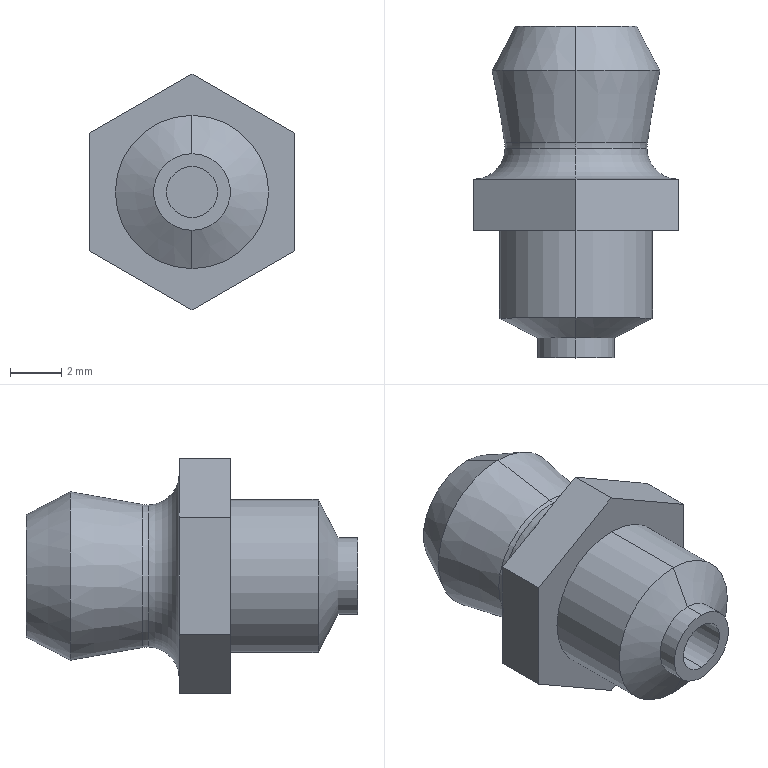Part | STEP file | JB/T7940.1-1995 straight-through grease cup 6 | 1 solid | 35 faces | box 8 x 13 x 9.238 mm | volume 360.504 mm3 | plane 17 | cylinder 8 | cone 6 | torus 4 | commonest cylinder face diameters 2 x4 3 x2 6 x2
STEP:
#1=CARTESIAN_POINT('',(0.,8.43,2.8));
#2=VERTEX_POINT('',#1);
#3=CARTESIAN_POINT('',(0.,8.218,2.782));
#4=VERTEX_POINT('',#3);
#5=CARTESIAN_POINT('',(0.,8.218,4.));
#6=DIRECTION('',(-1.,0.,0.));
#7=DIRECTION('',(0.,0.,1.));
#8=AXIS2_PLACEMENT_3D('',#5,#6,#7);
#9=CIRCLE('',#8,1.218);
#10=EDGE_CURVE('',#2,#4,#9,.T.);
#11=ORIENTED_EDGE('',*,*,#10,.T.);
#12=CARTESIAN_POINT('',(0.,8.218,-2.782));
#13=VERTEX_POINT('',#12);
#14=CARTESIAN_POINT('',(0.,8.218,0.));
#15=DIRECTION('',(0.,1.,0.));
#16=DIRECTION('',(0.,0.,1.));
#17=AXIS2_PLACEMENT_3D('',#14,#15,#16);
#18=CIRCLE('',#17,2.782);
#19=EDGE_CURVE('',#4,#13,#18,.T.);
#20=ORIENTED_EDGE('',*,*,#19,.T.);
#21=CARTESIAN_POINT('',(0.,8.43,-2.8));
#22=VERTEX_POINT('',#21);
#23=CARTESIAN_POINT('',(0.,8.218,-4.));
#24=DIRECTION('',(1.,0.,0.));
#25=DIRECTION('',(0.,0.,-1.));
#26=AXIS2_PLACEMENT_3D('',#23,#24,#25);
#27=CIRCLE('',#26,1.218);
#28=EDGE_CURVE('',#22,#13,#27,.T.);
#29=ORIENTED_EDGE('',*,*,#28,.F.);
#30=CARTESIAN_POINT('',(0.,8.43,0.));
#31=DIRECTION('',(0.,1.,0.));
#32=DIRECTION('',(0.,0.,1.));
#33=AXIS2_PLACEMENT_3D('',#30,#31,#32);
#34=CIRCLE('',#33,2.8);
#35=EDGE_CURVE('',#2,#22,#34,.T.);
#36=ORIENTED_EDGE('',*,*,#35,.F.);
#37=EDGE_LOOP('',(#11,#20,#29,#36));
#38=FACE_OUTER_BOUND('',#37,.T.);
#39=CARTESIAN_POINT('',(0.,8.218,0.));
#40=DIRECTION('',(0.,1.,0.));
#41=DIRECTION('',(0.,0.,1.));
#42=AXIS2_PLACEMENT_3D('',#39,#40,#41);
#43=TOROIDAL_SURFACE('',#42,4.,1.218);
#44=ADVANCED_FACE('',(#38),#43,.F.);
#45=ORIENTED_EDGE('',*,*,#28,.T.);
#46=CARTESIAN_POINT('',(0.,8.218,0.));
#47=DIRECTION('',(0.,1.,0.));
#48=DIRECTION('',(0.,0.,1.));
#49=AXIS2_PLACEMENT_3D('',#46,#47,#48);
#50=CIRCLE('',#49,2.782);
#51=EDGE_CURVE('',#13,#4,#50,.T.);
#52=ORIENTED_EDGE('',*,*,#51,.T.);
#53=ORIENTED_EDGE('',*,*,#10,.F.);
#54=CARTESIAN_POINT('',(0.,8.43,0.));
#55=DIRECTION('',(0.,1.,0.));
#56=DIRECTION('',(0.,0.,1.));
#57=AXIS2_PLACEMENT_3D('',#54,#55,#56);
#58=CIRCLE('',#57,2.8);
#59=EDGE_CURVE('',#22,#2,#58,.T.);
#60=ORIENTED_EDGE('',*,*,#59,.F.);
#61=EDGE_LOOP('',(#45,#52,#53,#60));
#62=FACE_OUTER_BOUND('',#61,.T.);
#63=CARTESIAN_POINT('',(0.,8.218,0.));
#64=DIRECTION('',(0.,1.,0.));
#65=DIRECTION('',(0.,0.,1.));
#66=AXIS2_PLACEMENT_3D('',#63,#64,#65);
#67=TOROIDAL_SURFACE('',#66,4.,1.218);
#68=ADVANCED_FACE('',(#62),#67,.F.);
#69=ORIENTED_EDGE('',*,*,#51,.F.);
#70=CARTESIAN_POINT('',(0.,7.,-4.));
#71=VERTEX_POINT('',#70);
#72=CARTESIAN_POINT('',(0.,8.218,-4.));
#73=DIRECTION('',(1.,0.,0.));
#74=DIRECTION('',(0.,0.,-1.));
#75=AXIS2_PLACEMENT_3D('',#72,#73,#74);
#76=CIRCLE('',#75,1.218);
#77=EDGE_CURVE('',#13,#71,#76,.T.);
#78=ORIENTED_EDGE('',*,*,#77,.T.);
#79=CARTESIAN_POINT('',(-2.,7.,-3.464));
#80=VERTEX_POINT('',#79);
#81=CARTESIAN_POINT('',(0.,7.,0.));
#82=DIRECTION('',(0.,1.,0.));
#83=DIRECTION('',(0.,0.,1.));
#84=AXIS2_PLACEMENT_3D('',#81,#82,#83);
#85=CIRCLE('',#84,4.);
#86=EDGE_CURVE('',#71,#80,#85,.T.);
#87=ORIENTED_EDGE('',*,*,#86,.T.);
#88=CARTESIAN_POINT('',(-4.,7.,0.));
#89=VERTEX_POINT('',#88);
#90=CARTESIAN_POINT('',(0.,7.,0.));
#91=DIRECTION('',(0.,1.,0.));
#92=DIRECTION('',(0.,0.,1.));
#93=AXIS2_PLACEMENT_3D('',#90,#91,#92);
#94=CIRCLE('',#93,4.);
#95=EDGE_CURVE('',#80,#89,#94,.T.);
#96=ORIENTED_EDGE('',*,*,#95,.T.);
#97=CARTESIAN_POINT('',(-2.,7.,3.464));
#98=VERTEX_POINT('',#97);
#99=CARTESIAN_POINT('',(0.,7.,0.));
#100=DIRECTION('',(0.,1.,0.));
#101=DIRECTION('',(0.,0.,1.));
#102=AXIS2_PLACEMENT_3D('',#99,#100,#101);
#103=CIRCLE('',#102,4.);
#104=EDGE_CURVE('',#89,#98,#103,.T.);
#105=ORIENTED_EDGE('',*,*,#104,.T.);
#106=CARTESIAN_POINT('',(0.,7.,4.));
#107=VERTEX_POINT('',#106);
#108=CARTESIAN_POINT('',(0.,7.,0.));
#109=DIRECTION('',(0.,1.,0.));
#110=DIRECTION('',(0.,0.,1.));
#111=AXIS2_PLACEMENT_3D('',#108,#109,#110);
#112=CIRCLE('',#111,4.);
#113=EDGE_CURVE('',#98,#107,#112,.T.);
#114=ORIENTED_EDGE('',*,*,#113,.T.);
#115=CARTESIAN_POINT('',(0.,8.218,4.));
#116=DIRECTION('',(-1.,0.,0.));
#117=DIRECTION('',(0.,0.,1.));
#118=AXIS2_PLACEMENT_3D('',#115,#116,#117);
#119=CIRCLE('',#118,1.218);
#120=EDGE_CURVE('',#4,#107,#119,.T.);
#121=ORIENTED_EDGE('',*,*,#120,.F.);
#122=EDGE_LOOP('',(#69,#78,#87,#96,#105,#114,#121));
#123=FACE_OUTER_BOUND('',#122,.T.);
#124=CARTESIAN_POINT('',(0.,8.218,0.));
#125=DIRECTION('',(0.,1.,0.));
#126=DIRECTION('',(0.,0.,1.));
#127=AXIS2_PLACEMENT_3D('',#124,#125,#126);
#128=TOROIDAL_SURFACE('',#127,4.,1.218);
#129=ADVANCED_FACE('',(#123),#128,.F.);
#130=ORIENTED_EDGE('',*,*,#35,.T.);
#131=CARTESIAN_POINT('',(0.,11.271,-3.3));
#132=VERTEX_POINT('',#131);
#133=CARTESIAN_POINT('',(0.,11.271,-3.3));
#134=DIRECTION('',(0.,0.9849,-0.1733));
#135=VECTOR('',#134,1000.);
#136=LINE('',#133,#135);
#137=EDGE_CURVE('',#22,#132,#136,.T.);
#138=ORIENTED_EDGE('',*,*,#137,.T.);
#139=CARTESIAN_POINT('',(0.,11.271,3.3));
#140=VERTEX_POINT('',#139);
#141=CARTESIAN_POINT('',(0.,11.271,0.));
#142=DIRECTION('',(0.,1.,0.));
#143=DIRECTION('',(0.,0.,1.));
#144=AXIS2_PLACEMENT_3D('',#141,#142,#143);
#145=CIRCLE('',#144,3.3);
#146=EDGE_CURVE('',#140,#132,#145,.T.);
#147=ORIENTED_EDGE('',*,*,#146,.F.);
#148=CARTESIAN_POINT('',(0.,11.271,3.3));
#149=DIRECTION('',(0.,0.9849,0.1733));
#150=VECTOR('',#149,1000.);
#151=LINE('',#148,#150);
#152=EDGE_CURVE('',#2,#140,#151,.T.);
#153=ORIENTED_EDGE('',*,*,#152,.F.);
#154=EDGE_LOOP('',(#130,#138,#147,#153));
#155=FACE_OUTER_BOUND('',#154,.T.);
#156=CARTESIAN_POINT('',(0.,11.271,0.));
#157=DIRECTION('',(0.,1.,0.));
#158=DIRECTION('',(0.,0.,1.));
#159=AXIS2_PLACEMENT_3D('',#156,#157,#158);
#160=CONICAL_SURFACE('',#159,3.3,0.1742);
#161=ADVANCED_FACE('',(#155),#160,.T.);
#162=CARTESIAN_POINT('',(0.,13.,2.4));
#163=VERTEX_POINT('',#162);
#164=CARTESIAN_POINT('',(0.,13.,-2.4));
#165=VERTEX_POINT('',#164);
#166=CARTESIAN_POINT('',(0.,13.,0.));
#167=DIRECTION('',(0.,1.,0.));
#168=DIRECTION('',(0.,0.,1.));
#169=AXIS2_PLACEMENT_3D('',#166,#167,#168);
#170=CIRCLE('',#169,2.4);
#171=EDGE_CURVE('',#163,#165,#170,.T.);
#172=ORIENTED_EDGE('',*,*,#171,.F.);
#173=CARTESIAN_POINT('',(0.,13.,2.4));
#174=DIRECTION('',(0.,-0.887,0.4617));
#175=VECTOR('',#174,1000.);
#176=LINE('',#173,#175);
#177=EDGE_CURVE('',#163,#140,#176,.T.);
#178=ORIENTED_EDGE('',*,*,#177,.T.);
#179=ORIENTED_EDGE('',*,*,#146,.T.);
#180=CARTESIAN_POINT('',(0.,13.,-2.4));
#181=DIRECTION('',(0.,-0.887,-0.4617));
#182=VECTOR('',#181,1000.);
#183=LINE('',#180,#182);
#184=EDGE_CURVE('',#165,#132,#183,.T.);
#185=ORIENTED_EDGE('',*,*,#184,.F.);
#186=EDGE_LOOP('',(#172,#178,#179,#185));
#187=FACE_OUTER_BOUND('',#186,.T.);
#188=CARTESIAN_POINT('',(0.,13.,0.));
#189=DIRECTION('',(0.,-1.,0.));
#190=DIRECTION('',(0.,0.,-1.));
#191=AXIS2_PLACEMENT_3D('',#188,#189,#190);
#192=CONICAL_SURFACE('',#191,2.4,0.48);
#193=ADVANCED_FACE('',(#187),#192,.T.);
#194=CARTESIAN_POINT('',(0.,7.,-1.));
#195=VERTEX_POINT('',#194);
#196=CARTESIAN_POINT('',(0.,7.,1.));
#197=VERTEX_POINT('',#196);
#198=CARTESIAN_POINT('',(0.,7.,0.));
#199=DIRECTION('',(0.,1.,0.));
#200=DIRECTION('',(0.,0.,1.));
#201=AXIS2_PLACEMENT_3D('',#198,#199,#200);
#202=CIRCLE('',#201,1.);
#203=EDGE_CURVE('',#195,#197,#202,.T.);
#204=ORIENTED_EDGE('',*,*,#203,.F.);
#205=CARTESIAN_POINT('',(0.,13.,-1.));
#206=VERTEX_POINT('',#205);
#207=CARTESIAN_POINT('',(0.,0.,-1.));
#208=DIRECTION('',(0.,1.,0.));
#209=VECTOR('',#208,1000.);
#210=LINE('',#207,#209);
#211=EDGE_CURVE('',#195,#206,#210,.T.);
#212=ORIENTED_EDGE('',*,*,#211,.T.);
#213=CARTESIAN_POINT('',(0.,13.,1.));
#214=VERTEX_POINT('',#213);
#215=CARTESIAN_POINT('',(0.,13.,0.));
#216=DIRECTION('',(0.,1.,0.));
#217=DIRECTION('',(0.,0.,1.));
#218=AXIS2_PLACEMENT_3D('',#215,#216,#217);
#219=CIRCLE('',#218,1.);
#220=EDGE_CURVE('',#206,#214,#219,.T.);
#221=ORIENTED_EDGE('',*,*,#220,.T.);
#222=CARTESIAN_POINT('',(0.,0.,1.));
#223=DIRECTION('',(0.,1.,0.));
#224=VECTOR('',#223,1000.);
#225=LINE('',#222,#224);
#226=EDGE_CURVE('',#197,#214,#225,.T.);
#227=ORIENTED_EDGE('',*,*,#226,.F.);
#228=EDGE_LOOP('',(#204,#212,#221,#227));
#229=FACE_OUTER_BOUND('',#228,.T.);
#230=CARTESIAN_POINT('',(0.,0.,0.));
#231=DIRECTION('',(0.,1.,0.));
#232=DIRECTION('',(0.,0.,1.));
#233=AXIS2_PLACEMENT_3D('',#230,#231,#232);
#234=CYLINDRICAL_SURFACE('',#233,1.);
#235=ADVANCED_FACE('',(#229),#234,.F.);
#236=CARTESIAN_POINT('',(0.,0.,1.5));
#237=VERTEX_POINT('',#236);
#238=CARTESIAN_POINT('',(0.,0.,-1.5));
#239=VERTEX_POINT('',#238);
#240=CARTESIAN_POINT('',(0.,0.,0.));
#241=DIRECTION('',(0.,1.,0.));
#242=DIRECTION('',(0.,0.,1.));
#243=AXIS2_PLACEMENT_3D('',#240,#241,#242);
#244=CIRCLE('',#243,1.5);
#245=EDGE_CURVE('',#237,#239,#244,.T.);
#246=ORIENTED_EDGE('',*,*,#245,.T.);
#247=CARTESIAN_POINT('',(0.,0.7809,-1.5));
#248=VERTEX_POINT('',#247);
#249=CARTESIAN_POINT('',(0.,0.,-1.5));
#250=DIRECTION('',(0.,1.,0.));
#251=VECTOR('',#250,1000.);
#252=LINE('',#249,#251);
#253=EDGE_CURVE('',#239,#248,#252,.T.);
#254=ORIENTED_EDGE('',*,*,#253,.T.);
#255=CARTESIAN_POINT('',(0.,0.7809,1.5));
#256=VERTEX_POINT('',#255);
#257=CARTESIAN_POINT('',(0.,0.7809,0.));
#258=DIRECTION('',(0.,1.,0.));
#259=DIRECTION('',(0.,0.,1.));
#260=AXIS2_PLACEMENT_3D('',#257,#258,#259);
#261=CIRCLE('',#260,1.5);
#262=EDGE_CURVE('',#256,#248,#261,.T.);
#263=ORIENTED_EDGE('',*,*,#262,.F.);
#264=CARTESIAN_POINT('',(0.,0.,1.5));
#265=DIRECTION('',(0.,1.,0.));
#266=VECTOR('',#265,1000.);
#267=LINE('',#264,#266);
#268=EDGE_CURVE('',#237,#256,#267,.T.);
#269=ORIENTED_EDGE('',*,*,#268,.F.);
#270=EDGE_LOOP('',(#246,#254,#263,#269));
#271=FACE_OUTER_BOUND('',#270,.T.);
#272=CARTESIAN_POINT('',(0.,0.,0.));
#273=DIRECTION('',(0.,1.,0.));
#274=DIRECTION('',(0.,0.,1.));
#275=AXIS2_PLACEMENT_3D('',#272,#273,#274);
#276=CYLINDRICAL_SURFACE('',#275,1.5);
#277=ADVANCED_FACE('',(#271),#276,.T.);
#278=ORIENTED_EDGE('',*,*,#262,.T.);
#279=CARTESIAN_POINT('',(0.,1.562,-3.));
#280=VERTEX_POINT('',#279);
#281=CARTESIAN_POINT('',(0.,1.562,-3.));
#282=DIRECTION('',(0.,0.4617,-0.887));
#283=VECTOR('',#282,1000.);
#284=LINE('',#281,#283);
#285=EDGE_CURVE('',#248,#280,#284,.T.);
#286=ORIENTED_EDGE('',*,*,#285,.T.);
#287=CARTESIAN_POINT('',(0.,1.562,3.));
#288=VERTEX_POINT('',#287);
#289=CARTESIAN_POINT('',(0.,1.562,0.));
#290=DIRECTION('',(0.,1.,0.));
#291=DIRECTION('',(0.,0.,1.));
#292=AXIS2_PLACEMENT_3D('',#289,#290,#291);
#293=CIRCLE('',#292,3.);
#294=EDGE_CURVE('',#288,#280,#293,.T.);
#295=ORIENTED_EDGE('',*,*,#294,.F.);
#296=CARTESIAN_POINT('',(0.,1.562,3.));
#297=DIRECTION('',(0.,0.4617,0.887));
#298=VECTOR('',#297,1000.);
#299=LINE('',#296,#298);
#300=EDGE_CURVE('',#256,#288,#299,.T.);
#301=ORIENTED_EDGE('',*,*,#300,.F.);
#302=EDGE_LOOP('',(#278,#286,#295,#301));
#303=FACE_OUTER_BOUND('',#302,.T.);
#304=CARTESIAN_POINT('',(0.,1.562,0.));
#305=DIRECTION('',(0.,1.,0.));
#306=DIRECTION('',(0.,0.,1.));
#307=AXIS2_PLACEMENT_3D('',#304,#305,#306);
#308=CONICAL_SURFACE('',#307,3.,1.091);
#309=ADVANCED_FACE('',(#303),#308,.T.);
#310=ORIENTED_EDGE('',*,*,#294,.T.);
#311=CARTESIAN_POINT('',(0.,5.,-3.));
#312=VERTEX_POINT('',#311);
#313=CARTESIAN_POINT('',(0.,0.,-3.));
#314=DIRECTION('',(0.,1.,0.));
#315=VECTOR('',#314,1000.);
#316=LINE('',#313,#315);
#317=EDGE_CURVE('',#280,#312,#316,.T.);
#318=ORIENTED_EDGE('',*,*,#317,.T.);
#319=CARTESIAN_POINT('',(0.,5.,3.));
#320=VERTEX_POINT('',#319);
#321=CARTESIAN_POINT('',(0.,5.,0.));
#322=DIRECTION('',(0.,1.,0.));
#323=DIRECTION('',(0.,0.,1.));
#324=AXIS2_PLACEMENT_3D('',#321,#322,#323);
#325=CIRCLE('',#324,3.);
#326=EDGE_CURVE('',#320,#312,#325,.T.);
#327=ORIENTED_EDGE('',*,*,#326,.F.);
#328=CARTESIAN_POINT('',(0.,0.,3.));
#329=DIRECTION('',(0.,1.,0.));
#330=VECTOR('',#329,1000.);
#331=LINE('',#328,#330);
#332=EDGE_CURVE('',#288,#320,#331,.T.);
#333=ORIENTED_EDGE('',*,*,#332,.F.);
#334=EDGE_LOOP('',(#310,#318,#327,#333));
#335=FACE_OUTER_BOUND('',#334,.T.);
#336=CARTESIAN_POINT('',(0.,0.,0.));
#337=DIRECTION('',(0.,1.,0.));
#338=DIRECTION('',(0.,0.,1.));
#339=AXIS2_PLACEMENT_3D('',#336,#337,#338);
#340=CYLINDRICAL_SURFACE('',#339,3.);
#341=ADVANCED_FACE('',(#335),#340,.T.);
#342=CARTESIAN_POINT('',(0.,0.,-1.));
#343=VERTEX_POINT('',#342);
#344=CARTESIAN_POINT('',(0.,0.,1.));
#345=VERTEX_POINT('',#344);
#346=CARTESIAN_POINT('',(0.,0.,0.));
#347=DIRECTION('',(0.,1.,0.));
#348=DIRECTION('',(0.,0.,1.));
#349=AXIS2_PLACEMENT_3D('',#346,#347,#348);
#350=CIRCLE('',#349,1.);
#351=EDGE_CURVE('',#343,#345,#350,.T.);
#352=ORIENTED_EDGE('',*,*,#351,.F.);
#353=CARTESIAN_POINT('',(0.,5.,-1.));
#354=VERTEX_POINT('',#353);
#355=CARTESIAN_POINT('',(0.,0.,-1.));
#356=DIRECTION('',(0.,1.,0.));
#357=VECTOR('',#356,1000.);
#358=LINE('',#355,#357);
#359=EDGE_CURVE('',#343,#354,#358,.T.);
#360=ORIENTED_EDGE('',*,*,#359,.T.);
#361=CARTESIAN_POINT('',(0.,5.,1.));
#362=VERTEX_POINT('',#361);
#363=CARTESIAN_POINT('',(0.,5.,0.));
#364=DIRECTION('',(0.,1.,0.));
#365=DIRECTION('',(0.,0.,1.));
#366=AXIS2_PLACEMENT_3D('',#363,#364,#365);
#367=CIRCLE('',#366,1.);
#368=EDGE_CURVE('',#354,#362,#367,.T.);
#369=ORIENTED_EDGE('',*,*,#368,.T.);
#370=CARTESIAN_POINT('',(0.,0.,1.));
#371=DIRECTION('',(0.,1.,0.));
#372=VECTOR('',#371,1000.);
#373=LINE('',#370,#372);
#374=EDGE_CURVE('',#345,#362,#373,.T.);
#375=ORIENTED_EDGE('',*,*,#374,.F.);
#376=EDGE_LOOP('',(#352,#360,#369,#375));
#377=FACE_OUTER_BOUND('',#376,.T.);
#378=CARTESIAN_POINT('',(0.,0.,0.));
#379=DIRECTION('',(0.,1.,0.));
#380=DIRECTION('',(0.,0.,1.));
#381=AXIS2_PLACEMENT_3D('',#378,#379,#380);
#382=CYLINDRICAL_SURFACE('',#381,1.);
#383=ADVANCED_FACE('',(#377),#382,.F.);
#384=ORIENTED_EDGE('',*,*,#359,.F.);
#385=CARTESIAN_POINT('',(0.,0.,0.));
#386=DIRECTION('',(0.,1.,0.));
#387=DIRECTION('',(0.,0.,1.));
#388=AXIS2_PLACEMENT_3D('',#385,#386,#387);
#389=CIRCLE('',#388,1.);
#390=EDGE_CURVE('',#345,#343,#389,.T.);
#391=ORIENTED_EDGE('',*,*,#390,.F.);
#392=ORIENTED_EDGE('',*,*,#374,.T.);
#393=CARTESIAN_POINT('',(0.,5.,0.));
#394=DIRECTION('',(0.,1.,0.));
#395=DIRECTION('',(0.,0.,1.));
#396=AXIS2_PLACEMENT_3D('',#393,#394,#395);
#397=CIRCLE('',#396,1.);
#398=EDGE_CURVE('',#362,#354,#397,.T.);
#399=ORIENTED_EDGE('',*,*,#398,.T.);
#400=EDGE_LOOP('',(#384,#391,#392,#399));
#401=FACE_OUTER_BOUND('',#400,.T.);
#402=CARTESIAN_POINT('',(0.,0.,0.));
#403=DIRECTION('',(0.,1.,0.));
#404=DIRECTION('',(0.,0.,1.));
#405=AXIS2_PLACEMENT_3D('',#402,#403,#404);
#406=CYLINDRICAL_SURFACE('',#405,1.);
#407=ADVANCED_FACE('',(#401),#406,.F.);
#408=ORIENTED_EDGE('',*,*,#326,.T.);
#409=CARTESIAN_POINT('',(0.,5.,0.));
#410=DIRECTION('',(0.,1.,0.));
#411=DIRECTION('',(0.,0.,1.));
#412=AXIS2_PLACEMENT_3D('',#409,#410,#411);
#413=CIRCLE('',#412,3.);
#414=EDGE_CURVE('',#312,#320,#413,.T.);
#415=ORIENTED_EDGE('',*,*,#414,.T.);
#416=EDGE_LOOP('',(#408,#415));
#417=FACE_BOUND('',#416,.T.);
#418=CARTESIAN_POINT('',(4.,5.,2.309));
#419=VERTEX_POINT('',#418);
#420=CARTESIAN_POINT('',(0.,5.,4.619));
#421=VERTEX_POINT('',#420);
#422=CARTESIAN_POINT('',(4.,5.,2.309));
#423=DIRECTION('',(-0.866,0.,0.5));
#424=VECTOR('',#423,1000.);
#425=LINE('',#422,#424);
#426=EDGE_CURVE('',#419,#421,#425,.T.);
#427=ORIENTED_EDGE('',*,*,#426,.T.);
#428=CARTESIAN_POINT('',(-4.,5.,2.309));
#429=VERTEX_POINT('',#428);
#430=CARTESIAN_POINT('',(0.,5.,4.619));
#431=DIRECTION('',(-0.866,0.,-0.5));
#432=VECTOR('',#431,1000.);
#433=LINE('',#430,#432);
#434=EDGE_CURVE('',#421,#429,#433,.T.);
#435=ORIENTED_EDGE('',*,*,#434,.T.);
#436=CARTESIAN_POINT('',(-4.,5.,-2.309));
#437=VERTEX_POINT('',#436);
#438=CARTESIAN_POINT('',(-4.,5.,2.309));
#439=DIRECTION('',(0.,0.,-1.));
#440=VECTOR('',#439,1000.);
#441=LINE('',#438,#440);
#442=EDGE_CURVE('',#429,#437,#441,.T.);
#443=ORIENTED_EDGE('',*,*,#442,.T.);
#444=CARTESIAN_POINT('',(0.,5.,-4.619));
#445=VERTEX_POINT('',#444);
#446=CARTESIAN_POINT('',(-4.,5.,-2.309));
#447=DIRECTION('',(0.866,0.,-0.5));
#448=VECTOR('',#447,1000.);
#449=LINE('',#446,#448);
#450=EDGE_CURVE('',#437,#445,#449,.T.);
#451=ORIENTED_EDGE('',*,*,#450,.T.);
#452=CARTESIAN_POINT('',(4.,5.,-2.309));
#453=VERTEX_POINT('',#452);
#454=CARTESIAN_POINT('',(0.,5.,-4.619));
#455=DIRECTION('',(0.866,0.,0.5));
#456=VECTOR('',#455,1000.);
#457=LINE('',#454,#456);
#458=EDGE_CURVE('',#445,#453,#457,.T.);
#459=ORIENTED_EDGE('',*,*,#458,.T.);
#460=CARTESIAN_POINT('',(4.,5.,-2.309));
#461=DIRECTION('',(0.,0.,1.));
#462=VECTOR('',#461,1000.);
#463=LINE('',#460,#462);
#464=EDGE_CURVE('',#453,#419,#463,.T.);
#465=ORIENTED_EDGE('',*,*,#464,.T.);
#466=EDGE_LOOP('',(#427,#435,#443,#451,#459,#465));
#467=FACE_OUTER_BOUND('',#466,.T.);
#468=CARTESIAN_POINT('',(-3.,5.,0.));
#469=DIRECTION('',(0.,-1.,0.));
#470=DIRECTION('',(0.,0.,-1.));
#471=AXIS2_PLACEMENT_3D('',#468,#469,#470);
#472=PLANE('',#471);
#473=ADVANCED_FACE('',(#417,#467),#472,.T.);
#474=ORIENTED_EDGE('',*,*,#317,.F.);
#475=CARTESIAN_POINT('',(0.,1.562,0.));
#476=DIRECTION('',(0.,1.,0.));
#477=DIRECTION('',(0.,0.,1.));
#478=AXIS2_PLACEMENT_3D('',#475,#476,#477);
#479=CIRCLE('',#478,3.);
#480=EDGE_CURVE('',#280,#288,#479,.T.);
#481=ORIENTED_EDGE('',*,*,#480,.T.);
#482=ORIENTED_EDGE('',*,*,#332,.T.);
#483=ORIENTED_EDGE('',*,*,#414,.F.);
#484=EDGE_LOOP('',(#474,#481,#482,#483));
#485=FACE_OUTER_BOUND('',#484,.T.);
#486=CARTESIAN_POINT('',(0.,0.,0.));
#487=DIRECTION('',(0.,1.,0.));
#488=DIRECTION('',(0.,0.,1.));
#489=AXIS2_PLACEMENT_3D('',#486,#487,#488);
#490=CYLINDRICAL_SURFACE('',#489,3.);
#491=ADVANCED_FACE('',(#485),#490,.T.);
#492=ORIENTED_EDGE('',*,*,#285,.F.);
#493=CARTESIAN_POINT('',(0.,0.7809,0.));
#494=DIRECTION('',(0.,1.,0.));
#495=DIRECTION('',(0.,0.,1.));
#496=AXIS2_PLACEMENT_3D('',#493,#494,#495);
#497=CIRCLE('',#496,1.5);
#498=EDGE_CURVE('',#248,#256,#497,.T.);
#499=ORIENTED_EDGE('',*,*,#498,.T.);
#500=ORIENTED_EDGE('',*,*,#300,.T.);
#501=ORIENTED_EDGE('',*,*,#480,.F.);
#502=EDGE_LOOP('',(#492,#499,#500,#501));
#503=FACE_OUTER_BOUND('',#502,.T.);
#504=CARTESIAN_POINT('',(0.,1.562,0.));
#505=DIRECTION('',(0.,1.,0.));
#506=DIRECTION('',(0.,0.,1.));
#507=AXIS2_PLACEMENT_3D('',#504,#505,#506);
#508=CONICAL_SURFACE('',#507,3.,1.091);
#509=ADVANCED_FACE('',(#503),#508,.T.);
#510=ORIENTED_EDGE('',*,*,#253,.F.);
#511=CARTESIAN_POINT('',(0.,0.,0.));
#512=DIRECTION('',(0.,1.,0.));
#513=DIRECTION('',(0.,0.,1.));
#514=AXIS2_PLACEMENT_3D('',#511,#512,#513);
#515=CIRCLE('',#514,1.5);
#516=EDGE_CURVE('',#239,#237,#515,.T.);
#517=ORIENTED_EDGE('',*,*,#516,.T.);
#518=ORIENTED_EDGE('',*,*,#268,.T.);
#519=ORIENTED_EDGE('',*,*,#498,.F.);
#520=EDGE_LOOP('',(#510,#517,#518,#519));
#521=FACE_OUTER_BOUND('',#520,.T.);
#522=CARTESIAN_POINT('',(0.,0.,0.));
#523=DIRECTION('',(0.,1.,0.));
#524=DIRECTION('',(0.,0.,1.));
#525=AXIS2_PLACEMENT_3D('',#522,#523,#524);
#526=CYLINDRICAL_SURFACE('',#525,1.5);
#527=ADVANCED_FACE('',(#521),#526,.T.);
#528=ORIENTED_EDGE('',*,*,#390,.T.);
#529=ORIENTED_EDGE('',*,*,#351,.T.);
#530=EDGE_LOOP('',(#528,#529));
#531=FACE_BOUND('',#530,.T.);
#532=ORIENTED_EDGE('',*,*,#245,.F.);
#533=ORIENTED_EDGE('',*,*,#516,.F.);
#534=EDGE_LOOP('',(#532,#533));
#535=FACE_OUTER_BOUND('',#534,.T.);
#536=CARTESIAN_POINT('',(-1.,0.,0.));
#537=DIRECTION('',(0.,-1.,0.));
#538=DIRECTION('',(0.,0.,-1.));
#539=AXIS2_PLACEMENT_3D('',#536,#537,#538);
#540=PLANE('',#539);
#541=ADVANCED_FACE('',(#531,#535),#540,.T.);
#542=CARTESIAN_POINT('',(2.,7.,3.464));
#543=VERTEX_POINT('',#542);
#544=CARTESIAN_POINT('',(0.,7.,4.619));
#545=VERTEX_POINT('',#544);
#546=CARTESIAN_POINT('',(4.,7.,2.309));
#547=DIRECTION('',(-0.866,0.,0.5));
#548=VECTOR('',#547,1000.);
#549=LINE('',#546,#548);
#550=EDGE_CURVE('',#543,#545,#549,.T.);
#551=ORIENTED_EDGE('',*,*,#550,.F.);
#552=CARTESIAN_POINT('',(0.,7.,0.));
#553=DIRECTION('',(0.,1.,0.));
#554=DIRECTION('',(0.,0.,1.));
#555=AXIS2_PLACEMENT_3D('',#552,#553,#554);
#556=CIRCLE('',#555,4.);
#557=EDGE_CURVE('',#107,#543,#556,.T.);
#558=ORIENTED_EDGE('',*,*,#557,.F.);
#559=ORIENTED_EDGE('',*,*,#113,.F.);
#560=CARTESIAN_POINT('',(0.,7.,4.619));
#561=DIRECTION('',(-0.866,0.,-0.5));
#562=VECTOR('',#561,1000.);
#563=LINE('',#560,#562);
#564=EDGE_CURVE('',#545,#98,#563,.T.);
#565=ORIENTED_EDGE('',*,*,#564,.F.);
#566=EDGE_LOOP('',(#551,#558,#559,#565));
#567=FACE_OUTER_BOUND('',#566,.T.);
#568=CARTESIAN_POINT('',(4.,7.,6.928));
#569=DIRECTION('',(0.,1.,0.));
#570=DIRECTION('',(0.,0.,1.));
#571=AXIS2_PLACEMENT_3D('',#568,#569,#570);
#572=PLANE('',#571);
#573=ADVANCED_FACE('',(#567),#572,.T.);
#574=CARTESIAN_POINT('',(-4.,7.,-2.309));
#575=VERTEX_POINT('',#574);
#576=CARTESIAN_POINT('',(-4.,7.,-2.309));
#577=DIRECTION('',(0.,-1.,0.));
#578=VECTOR('',#577,1000.);
#579=LINE('',#576,#578);
#580=EDGE_CURVE('',#575,#437,#579,.T.);
#581=ORIENTED_EDGE('',*,*,#580,.T.);
#582=ORIENTED_EDGE('',*,*,#442,.F.);
#583=CARTESIAN_POINT('',(-4.,7.,2.309));
#584=VERTEX_POINT('',#583);
#585=CARTESIAN_POINT('',(-4.,7.,2.309));
#586=DIRECTION('',(0.,-1.,0.));
#587=VECTOR('',#586,1000.);
#588=LINE('',#585,#587);
#589=EDGE_CURVE('',#584,#429,#588,.T.);
#590=ORIENTED_EDGE('',*,*,#589,.F.);
#591=CARTESIAN_POINT('',(-4.,7.,2.309));
#592=DIRECTION('',(0.,0.,-1.));
#593=VECTOR('',#592,1000.);
#594=LINE('',#591,#593);
#595=EDGE_CURVE('',#584,#89,#594,.T.);
#596=ORIENTED_EDGE('',*,*,#595,.T.);
#597=CARTESIAN_POINT('',(-4.,7.,2.309));
#598=DIRECTION('',(0.,0.,-1.));
#599=VECTOR('',#598,1000.);
#600=LINE('',#597,#599);
#601=EDGE_CURVE('',#89,#575,#600,.T.);
#602=ORIENTED_EDGE('',*,*,#601,.T.);
#603=EDGE_LOOP('',(#581,#582,#590,#596,#602));
#604=FACE_OUTER_BOUND('',#603,.T.);
#605=CARTESIAN_POINT('',(-4.,7.,2.309));
#606=DIRECTION('',(-1.,0.,0.));
#607=DIRECTION('',(0.,0.,1.));
#608=AXIS2_PLACEMENT_3D('',#605,#606,#607);
#609=PLANE('',#608);
#610=ADVANCED_FACE('',(#604),#609,.T.);
#611=CARTESIAN_POINT('',(0.,7.,-4.619));
#612=VERTEX_POINT('',#611);
#613=CARTESIAN_POINT('',(0.,7.,-4.619));
#614=DIRECTION('',(0.,-1.,0.));
#615=VECTOR('',#614,1000.);
#616=LINE('',#613,#615);
#617=EDGE_CURVE('',#612,#445,#616,.T.);
#618=ORIENTED_EDGE('',*,*,#617,.T.);
#619=ORIENTED_EDGE('',*,*,#450,.F.);
#620=ORIENTED_EDGE('',*,*,#580,.F.);
#621=CARTESIAN_POINT('',(-4.,7.,-2.309));
#622=DIRECTION('',(0.866,0.,-0.5));
#623=VECTOR('',#622,1000.);
#624=LINE('',#621,#623);
#625=EDGE_CURVE('',#575,#80,#624,.T.);
#626=ORIENTED_EDGE('',*,*,#625,.T.);
#627=CARTESIAN_POINT('',(-4.,7.,-2.309));
#628=DIRECTION('',(0.866,0.,-0.5));
#629=VECTOR('',#628,1000.);
#630=LINE('',#627,#629);
#631=EDGE_CURVE('',#80,#612,#630,.T.);
#632=ORIENTED_EDGE('',*,*,#631,.T.);
#633=EDGE_LOOP('',(#618,#619,#620,#626,#632));
#634=FACE_OUTER_BOUND('',#633,.T.);
#635=CARTESIAN_POINT('',(-4.,7.,-2.309));
#636=DIRECTION('',(-0.5,0.,-0.866));
#637=DIRECTION('',(-0.866,0.,0.5));
#638=AXIS2_PLACEMENT_3D('',#635,#636,#637);
#639=PLANE('',#638);
#640=ADVANCED_FACE('',(#634),#639,.T.);
#641=CARTESIAN_POINT('',(4.,7.,-2.309));
#642=VERTEX_POINT('',#641);
#643=CARTESIAN_POINT('',(4.,7.,-2.309));
#644=DIRECTION('',(0.,-1.,0.));
#645=VECTOR('',#644,1000.);
#646=LINE('',#643,#645);
#647=EDGE_CURVE('',#642,#453,#646,.T.);
#648=ORIENTED_EDGE('',*,*,#647,.T.);
#649=ORIENTED_EDGE('',*,*,#458,.F.);
#650=ORIENTED_EDGE('',*,*,#617,.F.);
#651=CARTESIAN_POINT('',(2.,7.,-3.464));
#652=VERTEX_POINT('',#651);
#653=CARTESIAN_POINT('',(0.,7.,-4.619));
#654=DIRECTION('',(0.866,0.,0.5));
#655=VECTOR('',#654,1000.);
#656=LINE('',#653,#655);
#657=EDGE_CURVE('',#612,#652,#656,.T.);
#658=ORIENTED_EDGE('',*,*,#657,.T.);
#659=CARTESIAN_POINT('',(0.,7.,-4.619));
#660=DIRECTION('',(0.866,0.,0.5));
#661=VECTOR('',#660,1000.);
#662=LINE('',#659,#661);
#663=EDGE_CURVE('',#652,#642,#662,.T.);
#664=ORIENTED_EDGE('',*,*,#663,.T.);
#665=EDGE_LOOP('',(#648,#649,#650,#658,#664));
#666=FACE_OUTER_BOUND('',#665,.T.);
#667=CARTESIAN_POINT('',(0.,7.,-4.619));
#668=DIRECTION('',(0.5,0.,-0.866));
#669=DIRECTION('',(-0.866,0.,-0.5));
#670=AXIS2_PLACEMENT_3D('',#667,#668,#669);
#671=PLANE('',#670);
#672=ADVANCED_FACE('',(#666),#671,.T.);
#673=CARTESIAN_POINT('',(4.,7.,2.309));
#674=VERTEX_POINT('',#673);
#675=CARTESIAN_POINT('',(4.,7.,2.309));
#676=DIRECTION('',(0.,-1.,0.));
#677=VECTOR('',#676,1000.);
#678=LINE('',#675,#677);
#679=EDGE_CURVE('',#674,#419,#678,.T.);
#680=ORIENTED_EDGE('',*,*,#679,.T.);
#681=ORIENTED_EDGE('',*,*,#464,.F.);
#682=ORIENTED_EDGE('',*,*,#647,.F.);
#683=CARTESIAN_POINT('',(4.,7.,0.));
#684=VERTEX_POINT('',#683);
#685=CARTESIAN_POINT('',(4.,7.,-2.309));
#686=DIRECTION('',(0.,0.,1.));
#687=VECTOR('',#686,1000.);
#688=LINE('',#685,#687);
#689=EDGE_CURVE('',#642,#684,#688,.T.);
#690=ORIENTED_EDGE('',*,*,#689,.T.);
#691=CARTESIAN_POINT('',(4.,7.,-2.309));
#692=DIRECTION('',(0.,0.,1.));
#693=VECTOR('',#692,1000.);
#694=LINE('',#691,#693);
#695=EDGE_CURVE('',#684,#674,#694,.T.);
#696=ORIENTED_EDGE('',*,*,#695,.T.);
#697=EDGE_LOOP('',(#680,#681,#682,#690,#696));
#698=FACE_OUTER_BOUND('',#697,.T.);
#699=CARTESIAN_POINT('',(4.,7.,-2.309));
#700=DIRECTION('',(1.,0.,0.));
#701=DIRECTION('',(0.,0.,-1.));
#702=AXIS2_PLACEMENT_3D('',#699,#700,#701);
#703=PLANE('',#702);
#704=ADVANCED_FACE('',(#698),#703,.T.);
#705=CARTESIAN_POINT('',(0.,7.,4.619));
#706=DIRECTION('',(0.,-1.,0.));
#707=VECTOR('',#706,1000.);
#708=LINE('',#705,#707);
#709=EDGE_CURVE('',#545,#421,#708,.T.);
#710=ORIENTED_EDGE('',*,*,#709,.T.);
#711=ORIENTED_EDGE('',*,*,#426,.F.);
#712=ORIENTED_EDGE('',*,*,#679,.F.);
#713=CARTESIAN_POINT('',(4.,7.,2.309));
#714=DIRECTION('',(-0.866,0.,0.5));
#715=VECTOR('',#714,1000.);
#716=LINE('',#713,#715);
#717=EDGE_CURVE('',#674,#543,#716,.T.);
#718=ORIENTED_EDGE('',*,*,#717,.T.);
#719=ORIENTED_EDGE('',*,*,#550,.T.);
#720=EDGE_LOOP('',(#710,#711,#712,#718,#719));
#721=FACE_OUTER_BOUND('',#720,.T.);
#722=CARTESIAN_POINT('',(4.,7.,2.309));
#723=DIRECTION('',(0.5,0.,0.866));
#724=DIRECTION('',(0.866,0.,-0.5));
#725=AXIS2_PLACEMENT_3D('',#722,#723,#724);
#726=PLANE('',#725);
#727=ADVANCED_FACE('',(#721),#726,.T.);
#728=ORIENTED_EDGE('',*,*,#434,.F.);
#729=ORIENTED_EDGE('',*,*,#709,.F.);
#730=ORIENTED_EDGE('',*,*,#564,.T.);
#731=CARTESIAN_POINT('',(0.,7.,4.619));
#732=DIRECTION('',(-0.866,0.,-0.5));
#733=VECTOR('',#732,1000.);
#734=LINE('',#731,#733);
#735=EDGE_CURVE('',#98,#584,#734,.T.);
#736=ORIENTED_EDGE('',*,*,#735,.T.);
#737=ORIENTED_EDGE('',*,*,#589,.T.);
#738=EDGE_LOOP('',(#728,#729,#730,#736,#737));
#739=FACE_OUTER_BOUND('',#738,.T.);
#740=CARTESIAN_POINT('',(0.,7.,4.619));
#741=DIRECTION('',(-0.5,0.,0.866));
#742=DIRECTION('',(0.866,0.,0.5));
#743=AXIS2_PLACEMENT_3D('',#740,#741,#742);
#744=PLANE('',#743);
#745=ADVANCED_FACE('',(#739),#744,.T.);
#746=ORIENTED_EDGE('',*,*,#695,.F.);
#747=CARTESIAN_POINT('',(0.,7.,0.));
#748=DIRECTION('',(0.,1.,0.));
#749=DIRECTION('',(0.,0.,1.));
#750=AXIS2_PLACEMENT_3D('',#747,#748,#749);
#751=CIRCLE('',#750,4.);
#752=EDGE_CURVE('',#543,#684,#751,.T.);
#753=ORIENTED_EDGE('',*,*,#752,.F.);
#754=ORIENTED_EDGE('',*,*,#717,.F.);
#755=EDGE_LOOP('',(#746,#753,#754));
#756=FACE_OUTER_BOUND('',#755,.T.);
#757=CARTESIAN_POINT('',(4.,7.,6.928));
#758=DIRECTION('',(0.,1.,0.));
#759=DIRECTION('',(0.,0.,1.));
#760=AXIS2_PLACEMENT_3D('',#757,#758,#759);
#761=PLANE('',#760);
#762=ADVANCED_FACE('',(#756),#761,.T.);
#763=ORIENTED_EDGE('',*,*,#663,.F.);
#764=CARTESIAN_POINT('',(0.,7.,0.));
#765=DIRECTION('',(0.,1.,0.));
#766=DIRECTION('',(0.,0.,1.));
#767=AXIS2_PLACEMENT_3D('',#764,#765,#766);
#768=CIRCLE('',#767,4.);
#769=EDGE_CURVE('',#684,#652,#768,.T.);
#770=ORIENTED_EDGE('',*,*,#769,.F.);
#771=ORIENTED_EDGE('',*,*,#689,.F.);
#772=EDGE_LOOP('',(#763,#770,#771));
#773=FACE_OUTER_BOUND('',#772,.T.);
#774=CARTESIAN_POINT('',(4.,7.,6.928));
#775=DIRECTION('',(0.,1.,0.));
#776=DIRECTION('',(0.,0.,1.));
#777=AXIS2_PLACEMENT_3D('',#774,#775,#776);
#778=PLANE('',#777);
#779=ADVANCED_FACE('',(#773),#778,.T.);
#780=ORIENTED_EDGE('',*,*,#631,.F.);
#781=ORIENTED_EDGE('',*,*,#86,.F.);
#782=CARTESIAN_POINT('',(0.,7.,0.));
#783=DIRECTION('',(0.,1.,0.));
#784=DIRECTION('',(0.,0.,1.));
#785=AXIS2_PLACEMENT_3D('',#782,#783,#784);
#786=CIRCLE('',#785,4.);
#787=EDGE_CURVE('',#652,#71,#786,.T.);
#788=ORIENTED_EDGE('',*,*,#787,.F.);
#789=ORIENTED_EDGE('',*,*,#657,.F.);
#790=EDGE_LOOP('',(#780,#781,#788,#789));
#791=FACE_OUTER_BOUND('',#790,.T.);
#792=CARTESIAN_POINT('',(4.,7.,6.928));
#793=DIRECTION('',(0.,1.,0.));
#794=DIRECTION('',(0.,0.,1.));
#795=AXIS2_PLACEMENT_3D('',#792,#793,#794);
#796=PLANE('',#795);
#797=ADVANCED_FACE('',(#791),#796,.T.);
#798=ORIENTED_EDGE('',*,*,#601,.F.);
#799=ORIENTED_EDGE('',*,*,#95,.F.);
#800=ORIENTED_EDGE('',*,*,#625,.F.);
#801=EDGE_LOOP('',(#798,#799,#800));
#802=FACE_OUTER_BOUND('',#801,.T.);
#803=CARTESIAN_POINT('',(4.,7.,6.928));
#804=DIRECTION('',(0.,1.,0.));
#805=DIRECTION('',(0.,0.,1.));
#806=AXIS2_PLACEMENT_3D('',#803,#804,#805);
#807=PLANE('',#806);
#808=ADVANCED_FACE('',(#802),#807,.T.);
#809=ORIENTED_EDGE('',*,*,#735,.F.);
#810=ORIENTED_EDGE('',*,*,#104,.F.);
#811=ORIENTED_EDGE('',*,*,#595,.F.);
#812=EDGE_LOOP('',(#809,#810,#811));
#813=FACE_OUTER_BOUND('',#812,.T.);
#814=CARTESIAN_POINT('',(4.,7.,6.928));
#815=DIRECTION('',(0.,1.,0.));
#816=DIRECTION('',(0.,0.,1.));
#817=AXIS2_PLACEMENT_3D('',#814,#815,#816);
#818=PLANE('',#817);
#819=ADVANCED_FACE('',(#813),#818,.T.);
#820=CARTESIAN_POINT('',(0.,13.,0.));
#821=DIRECTION('',(0.,1.,0.));
#822=DIRECTION('',(0.,0.,1.));
#823=AXIS2_PLACEMENT_3D('',#820,#821,#822);
#824=CIRCLE('',#823,2.4);
#825=EDGE_CURVE('',#165,#163,#824,.T.);
#826=ORIENTED_EDGE('',*,*,#825,.T.);
#827=ORIENTED_EDGE('',*,*,#171,.T.);
#828=EDGE_LOOP('',(#826,#827));
#829=FACE_OUTER_BOUND('',#828,.T.);
#830=CARTESIAN_POINT('',(0.,13.,0.));
#831=DIRECTION('',(0.,1.,0.));
#832=DIRECTION('',(0.,0.,1.));
#833=AXIS2_PLACEMENT_3D('',#830,#831,#832);
#834=CIRCLE('',#833,1.);
#835=EDGE_CURVE('',#214,#206,#834,.T.);
#836=ORIENTED_EDGE('',*,*,#835,.F.);
#837=ORIENTED_EDGE('',*,*,#220,.F.);
#838=EDGE_LOOP('',(#836,#837));
#839=FACE_BOUND('',#838,.T.);
#840=CARTESIAN_POINT('',(-1.,13.,0.));
#841=DIRECTION('',(0.,1.,0.));
#842=DIRECTION('',(0.,0.,1.));
#843=AXIS2_PLACEMENT_3D('',#840,#841,#842);
#844=PLANE('',#843);
#845=ADVANCED_FACE('',(#829,#839),#844,.T.);
#846=ORIENTED_EDGE('',*,*,#211,.F.);
#847=CARTESIAN_POINT('',(0.,7.,0.));
#848=DIRECTION('',(0.,1.,0.));
#849=DIRECTION('',(0.,0.,1.));
#850=AXIS2_PLACEMENT_3D('',#847,#848,#849);
#851=CIRCLE('',#850,1.);
#852=EDGE_CURVE('',#197,#195,#851,.T.);
#853=ORIENTED_EDGE('',*,*,#852,.F.);
#854=ORIENTED_EDGE('',*,*,#226,.T.);
#855=ORIENTED_EDGE('',*,*,#835,.T.);
#856=EDGE_LOOP('',(#846,#853,#854,#855));
#857=FACE_OUTER_BOUND('',#856,.T.);
#858=CARTESIAN_POINT('',(0.,0.,0.));
#859=DIRECTION('',(0.,1.,0.));
#860=DIRECTION('',(0.,0.,1.));
#861=AXIS2_PLACEMENT_3D('',#858,#859,#860);
#862=CYLINDRICAL_SURFACE('',#861,1.);
#863=ADVANCED_FACE('',(#857),#862,.F.);
#864=ORIENTED_EDGE('',*,*,#177,.F.);
#865=ORIENTED_EDGE('',*,*,#825,.F.);
#866=ORIENTED_EDGE('',*,*,#184,.T.);
#867=CARTESIAN_POINT('',(0.,11.271,0.));
#868=DIRECTION('',(0.,1.,0.));
#869=DIRECTION('',(0.,0.,1.));
#870=AXIS2_PLACEMENT_3D('',#867,#868,#869);
#871=CIRCLE('',#870,3.3);
#872=EDGE_CURVE('',#132,#140,#871,.T.);
#873=ORIENTED_EDGE('',*,*,#872,.T.);
#874=EDGE_LOOP('',(#864,#865,#866,#873));
#875=FACE_OUTER_BOUND('',#874,.T.);
#876=CARTESIAN_POINT('',(0.,13.,0.));
#877=DIRECTION('',(0.,-1.,0.));
#878=DIRECTION('',(0.,0.,-1.));
#879=AXIS2_PLACEMENT_3D('',#876,#877,#878);
#880=CONICAL_SURFACE('',#879,2.4,0.48);
#881=ADVANCED_FACE('',(#875),#880,.T.);
#882=ORIENTED_EDGE('',*,*,#137,.F.);
#883=ORIENTED_EDGE('',*,*,#59,.T.);
#884=ORIENTED_EDGE('',*,*,#152,.T.);
#885=ORIENTED_EDGE('',*,*,#872,.F.);
#886=EDGE_LOOP('',(#882,#883,#884,#885));
#887=FACE_OUTER_BOUND('',#886,.T.);
#888=CARTESIAN_POINT('',(0.,11.271,0.));
#889=DIRECTION('',(0.,1.,0.));
#890=DIRECTION('',(0.,0.,1.));
#891=AXIS2_PLACEMENT_3D('',#888,#889,#890);
#892=CONICAL_SURFACE('',#891,3.3,0.1742);
#893=ADVANCED_FACE('',(#887),#892,.T.);
#894=ORIENTED_EDGE('',*,*,#19,.F.);
#895=ORIENTED_EDGE('',*,*,#120,.T.);
#896=ORIENTED_EDGE('',*,*,#557,.T.);
#897=ORIENTED_EDGE('',*,*,#752,.T.);
#898=ORIENTED_EDGE('',*,*,#769,.T.);
#899=ORIENTED_EDGE('',*,*,#787,.T.);
#900=ORIENTED_EDGE('',*,*,#77,.F.);
#901=EDGE_LOOP('',(#894,#895,#896,#897,#898,#899,#900));
#902=FACE_OUTER_BOUND('',#901,.T.);
#903=CARTESIAN_POINT('',(0.,8.218,0.));
#904=DIRECTION('',(0.,1.,0.));
#905=DIRECTION('',(0.,0.,1.));
#906=AXIS2_PLACEMENT_3D('',#903,#904,#905);
#907=TOROIDAL_SURFACE('',#906,4.,1.218);
#908=ADVANCED_FACE('',(#902),#907,.F.);
#909=ORIENTED_EDGE('',*,*,#398,.F.);
#910=ORIENTED_EDGE('',*,*,#368,.F.);
#911=EDGE_LOOP('',(#909,#910));
#912=FACE_OUTER_BOUND('',#911,.T.);
#913=CARTESIAN_POINT('',(4.,5.,6.928));
#914=DIRECTION('',(0.,1.,0.));
#915=DIRECTION('',(0.,0.,1.));
#916=AXIS2_PLACEMENT_3D('',#913,#914,#915);
#917=PLANE('',#916);
#918=ADVANCED_FACE('',(#912),#917,.F.);
#919=ORIENTED_EDGE('',*,*,#852,.T.);
#920=ORIENTED_EDGE('',*,*,#203,.T.);
#921=EDGE_LOOP('',(#919,#920));
#922=FACE_OUTER_BOUND('',#921,.T.);
#923=CARTESIAN_POINT('',(4.,7.,6.928));
#924=DIRECTION('',(0.,1.,0.));
#925=DIRECTION('',(0.,0.,1.));
#926=AXIS2_PLACEMENT_3D('',#923,#924,#925);
#927=PLANE('',#926);
#928=ADVANCED_FACE('',(#922),#927,.T.);
#929=CLOSED_SHELL('',(#44,#68,#129,#161,#193,#235,#277,#309,#341,#383,#407,#473,#491,#509,#527,#541,#573,#610,#640,#672,#704,#727,#745,#762,#779,#797,#808,#819,#845,#863,#881,#893,#908,#918,#928));
#930=MANIFOLD_SOLID_BREP('',#929);
#931=CARTESIAN_POINT('',(0.,0.,0.));
#932=DIRECTION('',(0.,0.,1.));
#933=DIRECTION('',(1.,0.,0.));
#934=AXIS2_PLACEMENT_3D('',#931,#932,#933);
#935=(LENGTH_UNIT()NAMED_UNIT(*)SI_UNIT(.MILLI.,.METRE.));
#936=UNCERTAINTY_MEASURE_WITH_UNIT(LENGTH_MEASURE(0.00001),#935,'','');
#937=(NAMED_UNIT(*)PLANE_ANGLE_UNIT()SI_UNIT($,.RADIAN.));
#938=(NAMED_UNIT(*)SI_UNIT($,.STERADIAN.)SOLID_ANGLE_UNIT());
#939=(GEOMETRIC_REPRESENTATION_CONTEXT(3)GLOBAL_UNCERTAINTY_ASSIGNED_CONTEXT((#936))GLOBAL_UNIT_ASSIGNED_CONTEXT((#935,#937,#938))REPRESENTATION_CONTEXT('',''));
#940=ADVANCED_BREP_SHAPE_REPRESENTATION('',(#930,#934),#939);